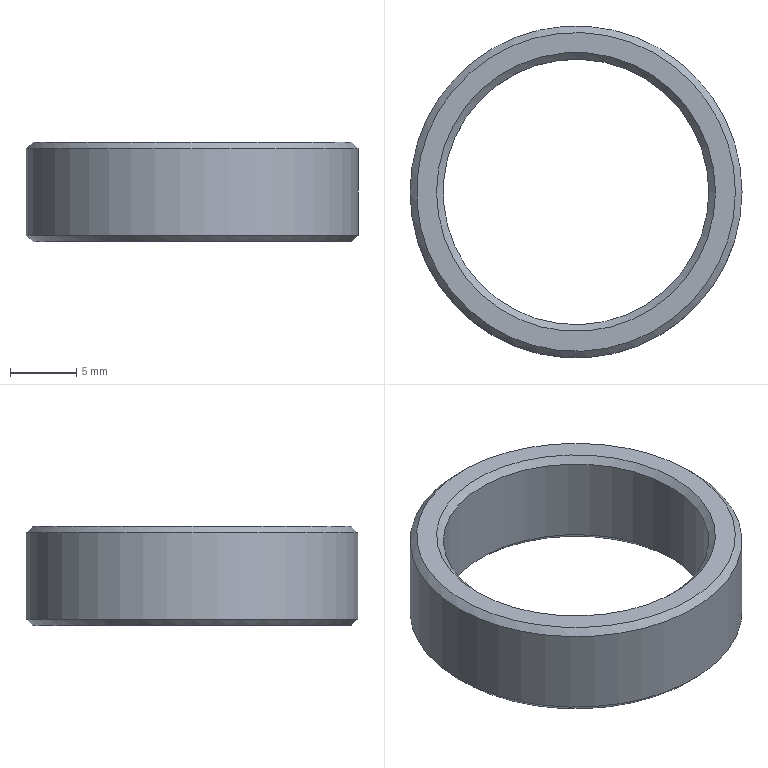Part | NX | features BREP 1 | 1 solid | 8 faces | box 25 x 25 x 7.5 mm | volume 1290 mm3 | cone 4 | cylinder 2 | plane 2 | commonest cylinder face diameters 20 x1 25 x1
STEP:
#1=CARTESIAN_POINT('',(12.5,0.,7.));
#2=VERTEX_POINT('',#1);
#3=CARTESIAN_POINT('',(0.,0.,7.));
#4=DIRECTION('',(0.,0.,-1.));
#5=DIRECTION('',(1.,0.,0.));
#6=AXIS2_PLACEMENT_3D('',#3,#4,#5);
#7=CIRCLE('',#6,12.5);
#8=EDGE_CURVE('',#2,#2,#7,.T.);
#9=ORIENTED_EDGE('',*,*,#8,.F.);
#10=EDGE_LOOP('',(#9));
#11=FACE_BOUND('',#10,.T.);
#12=CARTESIAN_POINT('',(12.,0.,7.5));
#13=VERTEX_POINT('',#12);
#14=CARTESIAN_POINT('',(0.,0.,7.5));
#15=DIRECTION('',(0.,0.,1.));
#16=DIRECTION('',(1.,0.,0.));
#17=AXIS2_PLACEMENT_3D('',#14,#15,#16);
#18=CIRCLE('',#17,12.);
#19=EDGE_CURVE('',#13,#13,#18,.T.);
#20=ORIENTED_EDGE('',*,*,#19,.F.);
#21=EDGE_LOOP('',(#20));
#22=FACE_BOUND('',#21,.T.);
#23=CARTESIAN_POINT('',(0.,0.,7.5));
#24=DIRECTION('',(0.,0.,-1.));
#25=DIRECTION('',(-1.,0.,0.));
#26=AXIS2_PLACEMENT_3D('',#23,#24,#25);
#27=CONICAL_SURFACE('',#26,12.,0.7854);
#28=ADVANCED_FACE('',(#11,#22),#27,.T.);
#29=CARTESIAN_POINT('',(12.5,0.,0.5));
#30=VERTEX_POINT('',#29);
#31=CARTESIAN_POINT('',(0.,0.,0.5));
#32=DIRECTION('',(0.,0.,1.));
#33=DIRECTION('',(1.,0.,0.));
#34=AXIS2_PLACEMENT_3D('',#31,#32,#33);
#35=CIRCLE('',#34,12.5);
#36=EDGE_CURVE('',#30,#30,#35,.T.);
#37=ORIENTED_EDGE('',*,*,#36,.F.);
#38=EDGE_LOOP('',(#37));
#39=FACE_BOUND('',#38,.T.);
#40=CARTESIAN_POINT('',(12.,0.,0.));
#41=VERTEX_POINT('',#40);
#42=CARTESIAN_POINT('',(0.,0.,0.));
#43=DIRECTION('',(0.,0.,-1.));
#44=DIRECTION('',(1.,0.,0.));
#45=AXIS2_PLACEMENT_3D('',#42,#43,#44);
#46=CIRCLE('',#45,12.);
#47=EDGE_CURVE('',#41,#41,#46,.T.);
#48=ORIENTED_EDGE('',*,*,#47,.F.);
#49=EDGE_LOOP('',(#48));
#50=FACE_BOUND('',#49,.T.);
#51=CARTESIAN_POINT('',(0.,0.,0.5));
#52=DIRECTION('',(0.,0.,1.));
#53=DIRECTION('',(1.,0.,0.));
#54=AXIS2_PLACEMENT_3D('',#51,#52,#53);
#55=CONICAL_SURFACE('',#54,12.5,0.7854);
#56=ADVANCED_FACE('',(#39,#50),#55,.T.);
#57=CARTESIAN_POINT('',(10.5,0.,7.5));
#58=VERTEX_POINT('',#57);
#59=CARTESIAN_POINT('',(0.,0.,7.5));
#60=DIRECTION('',(0.,0.,-1.));
#61=DIRECTION('',(1.,0.,0.));
#62=AXIS2_PLACEMENT_3D('',#59,#60,#61);
#63=CIRCLE('',#62,10.5);
#64=EDGE_CURVE('',#58,#58,#63,.T.);
#65=ORIENTED_EDGE('',*,*,#64,.F.);
#66=EDGE_LOOP('',(#65));
#67=FACE_BOUND('',#66,.T.);
#68=CARTESIAN_POINT('',(10.,0.,7.));
#69=VERTEX_POINT('',#68);
#70=CARTESIAN_POINT('',(0.,0.,7.));
#71=DIRECTION('',(0.,0.,1.));
#72=DIRECTION('',(1.,0.,0.));
#73=AXIS2_PLACEMENT_3D('',#70,#71,#72);
#74=CIRCLE('',#73,10.);
#75=EDGE_CURVE('',#69,#69,#74,.T.);
#76=ORIENTED_EDGE('',*,*,#75,.F.);
#77=EDGE_LOOP('',(#76));
#78=FACE_BOUND('',#77,.T.);
#79=CARTESIAN_POINT('',(0.,0.,7.));
#80=DIRECTION('',(0.,0.,1.));
#81=DIRECTION('',(1.,0.,0.));
#82=AXIS2_PLACEMENT_3D('',#79,#80,#81);
#83=CONICAL_SURFACE('',#82,10.,0.7854);
#84=ADVANCED_FACE('',(#67,#78),#83,.F.);
#85=CARTESIAN_POINT('',(10.5,0.,0.));
#86=VERTEX_POINT('',#85);
#87=CARTESIAN_POINT('',(0.,0.,0.));
#88=DIRECTION('',(0.,0.,1.));
#89=DIRECTION('',(1.,0.,0.));
#90=AXIS2_PLACEMENT_3D('',#87,#88,#89);
#91=CIRCLE('',#90,10.5);
#92=EDGE_CURVE('',#86,#86,#91,.T.);
#93=ORIENTED_EDGE('',*,*,#92,.F.);
#94=EDGE_LOOP('',(#93));
#95=FACE_BOUND('',#94,.T.);
#96=CARTESIAN_POINT('',(10.,0.,0.5));
#97=VERTEX_POINT('',#96);
#98=CARTESIAN_POINT('',(0.,0.,0.5));
#99=DIRECTION('',(0.,0.,-1.));
#100=DIRECTION('',(1.,0.,0.));
#101=AXIS2_PLACEMENT_3D('',#98,#99,#100);
#102=CIRCLE('',#101,10.);
#103=EDGE_CURVE('',#97,#97,#102,.T.);
#104=ORIENTED_EDGE('',*,*,#103,.F.);
#105=EDGE_LOOP('',(#104));
#106=FACE_BOUND('',#105,.T.);
#107=CARTESIAN_POINT('',(0.,0.,0.));
#108=DIRECTION('',(0.,0.,-1.));
#109=DIRECTION('',(-1.,0.,0.));
#110=AXIS2_PLACEMENT_3D('',#107,#108,#109);
#111=CONICAL_SURFACE('',#110,10.5,0.7854);
#112=ADVANCED_FACE('',(#95,#106),#111,.F.);
#113=ORIENTED_EDGE('',*,*,#103,.T.);
#114=EDGE_LOOP('',(#113));
#115=FACE_BOUND('',#114,.T.);
#116=ORIENTED_EDGE('',*,*,#75,.T.);
#117=EDGE_LOOP('',(#116));
#118=FACE_BOUND('',#117,.T.);
#119=CARTESIAN_POINT('',(0.,0.,7.5));
#120=DIRECTION('',(0.,0.,-1.));
#121=DIRECTION('',(-1.,0.,0.));
#122=AXIS2_PLACEMENT_3D('',#119,#120,#121);
#123=CYLINDRICAL_SURFACE('',#122,10.);
#124=ADVANCED_FACE('',(#115,#118),#123,.F.);
#125=ORIENTED_EDGE('',*,*,#36,.T.);
#126=EDGE_LOOP('',(#125));
#127=FACE_BOUND('',#126,.T.);
#128=ORIENTED_EDGE('',*,*,#8,.T.);
#129=EDGE_LOOP('',(#128));
#130=FACE_BOUND('',#129,.T.);
#131=CARTESIAN_POINT('',(0.,0.,7.5));
#132=DIRECTION('',(0.,0.,-1.));
#133=DIRECTION('',(-1.,0.,0.));
#134=AXIS2_PLACEMENT_3D('',#131,#132,#133);
#135=CYLINDRICAL_SURFACE('',#134,12.5);
#136=ADVANCED_FACE('',(#127,#130),#135,.T.);
#137=ORIENTED_EDGE('',*,*,#64,.T.);
#138=EDGE_LOOP('',(#137));
#139=FACE_BOUND('',#138,.T.);
#140=ORIENTED_EDGE('',*,*,#19,.T.);
#141=EDGE_LOOP('',(#140));
#142=FACE_BOUND('',#141,.T.);
#143=CARTESIAN_POINT('',(0.,0.,7.5));
#144=DIRECTION('',(0.,0.,1.));
#145=DIRECTION('',(1.,0.,0.));
#146=AXIS2_PLACEMENT_3D('',#143,#144,#145);
#147=PLANE('',#146);
#148=ADVANCED_FACE('',(#139,#142),#147,.T.);
#149=ORIENTED_EDGE('',*,*,#92,.T.);
#150=EDGE_LOOP('',(#149));
#151=FACE_BOUND('',#150,.T.);
#152=ORIENTED_EDGE('',*,*,#47,.T.);
#153=EDGE_LOOP('',(#152));
#154=FACE_BOUND('',#153,.T.);
#155=CARTESIAN_POINT('',(0.,0.,0.));
#156=DIRECTION('',(0.,0.,1.));
#157=DIRECTION('',(1.,0.,0.));
#158=AXIS2_PLACEMENT_3D('',#155,#156,#157);
#159=PLANE('',#158);
#160=ADVANCED_FACE('',(#151,#154),#159,.F.);
#161=CLOSED_SHELL('',(#28,#56,#84,#112,#124,#136,#148,#160));
#162=MANIFOLD_SOLID_BREP('',#161);
#163=(LENGTH_UNIT()NAMED_UNIT(*)SI_UNIT(.MILLI.,.METRE.));
#164=UNCERTAINTY_MEASURE_WITH_UNIT(LENGTH_MEASURE(0.00001),#163,'','');
#165=(NAMED_UNIT(*)PLANE_ANGLE_UNIT()SI_UNIT($,.RADIAN.));
#166=(NAMED_UNIT(*)SI_UNIT($,.STERADIAN.)SOLID_ANGLE_UNIT());
#167=(GEOMETRIC_REPRESENTATION_CONTEXT(3)GLOBAL_UNCERTAINTY_ASSIGNED_CONTEXT((#164))GLOBAL_UNIT_ASSIGNED_CONTEXT((#163,#165,#166))REPRESENTATION_CONTEXT('',''));
#168=ADVANCED_BREP_SHAPE_REPRESENTATION('',(#162),#167);